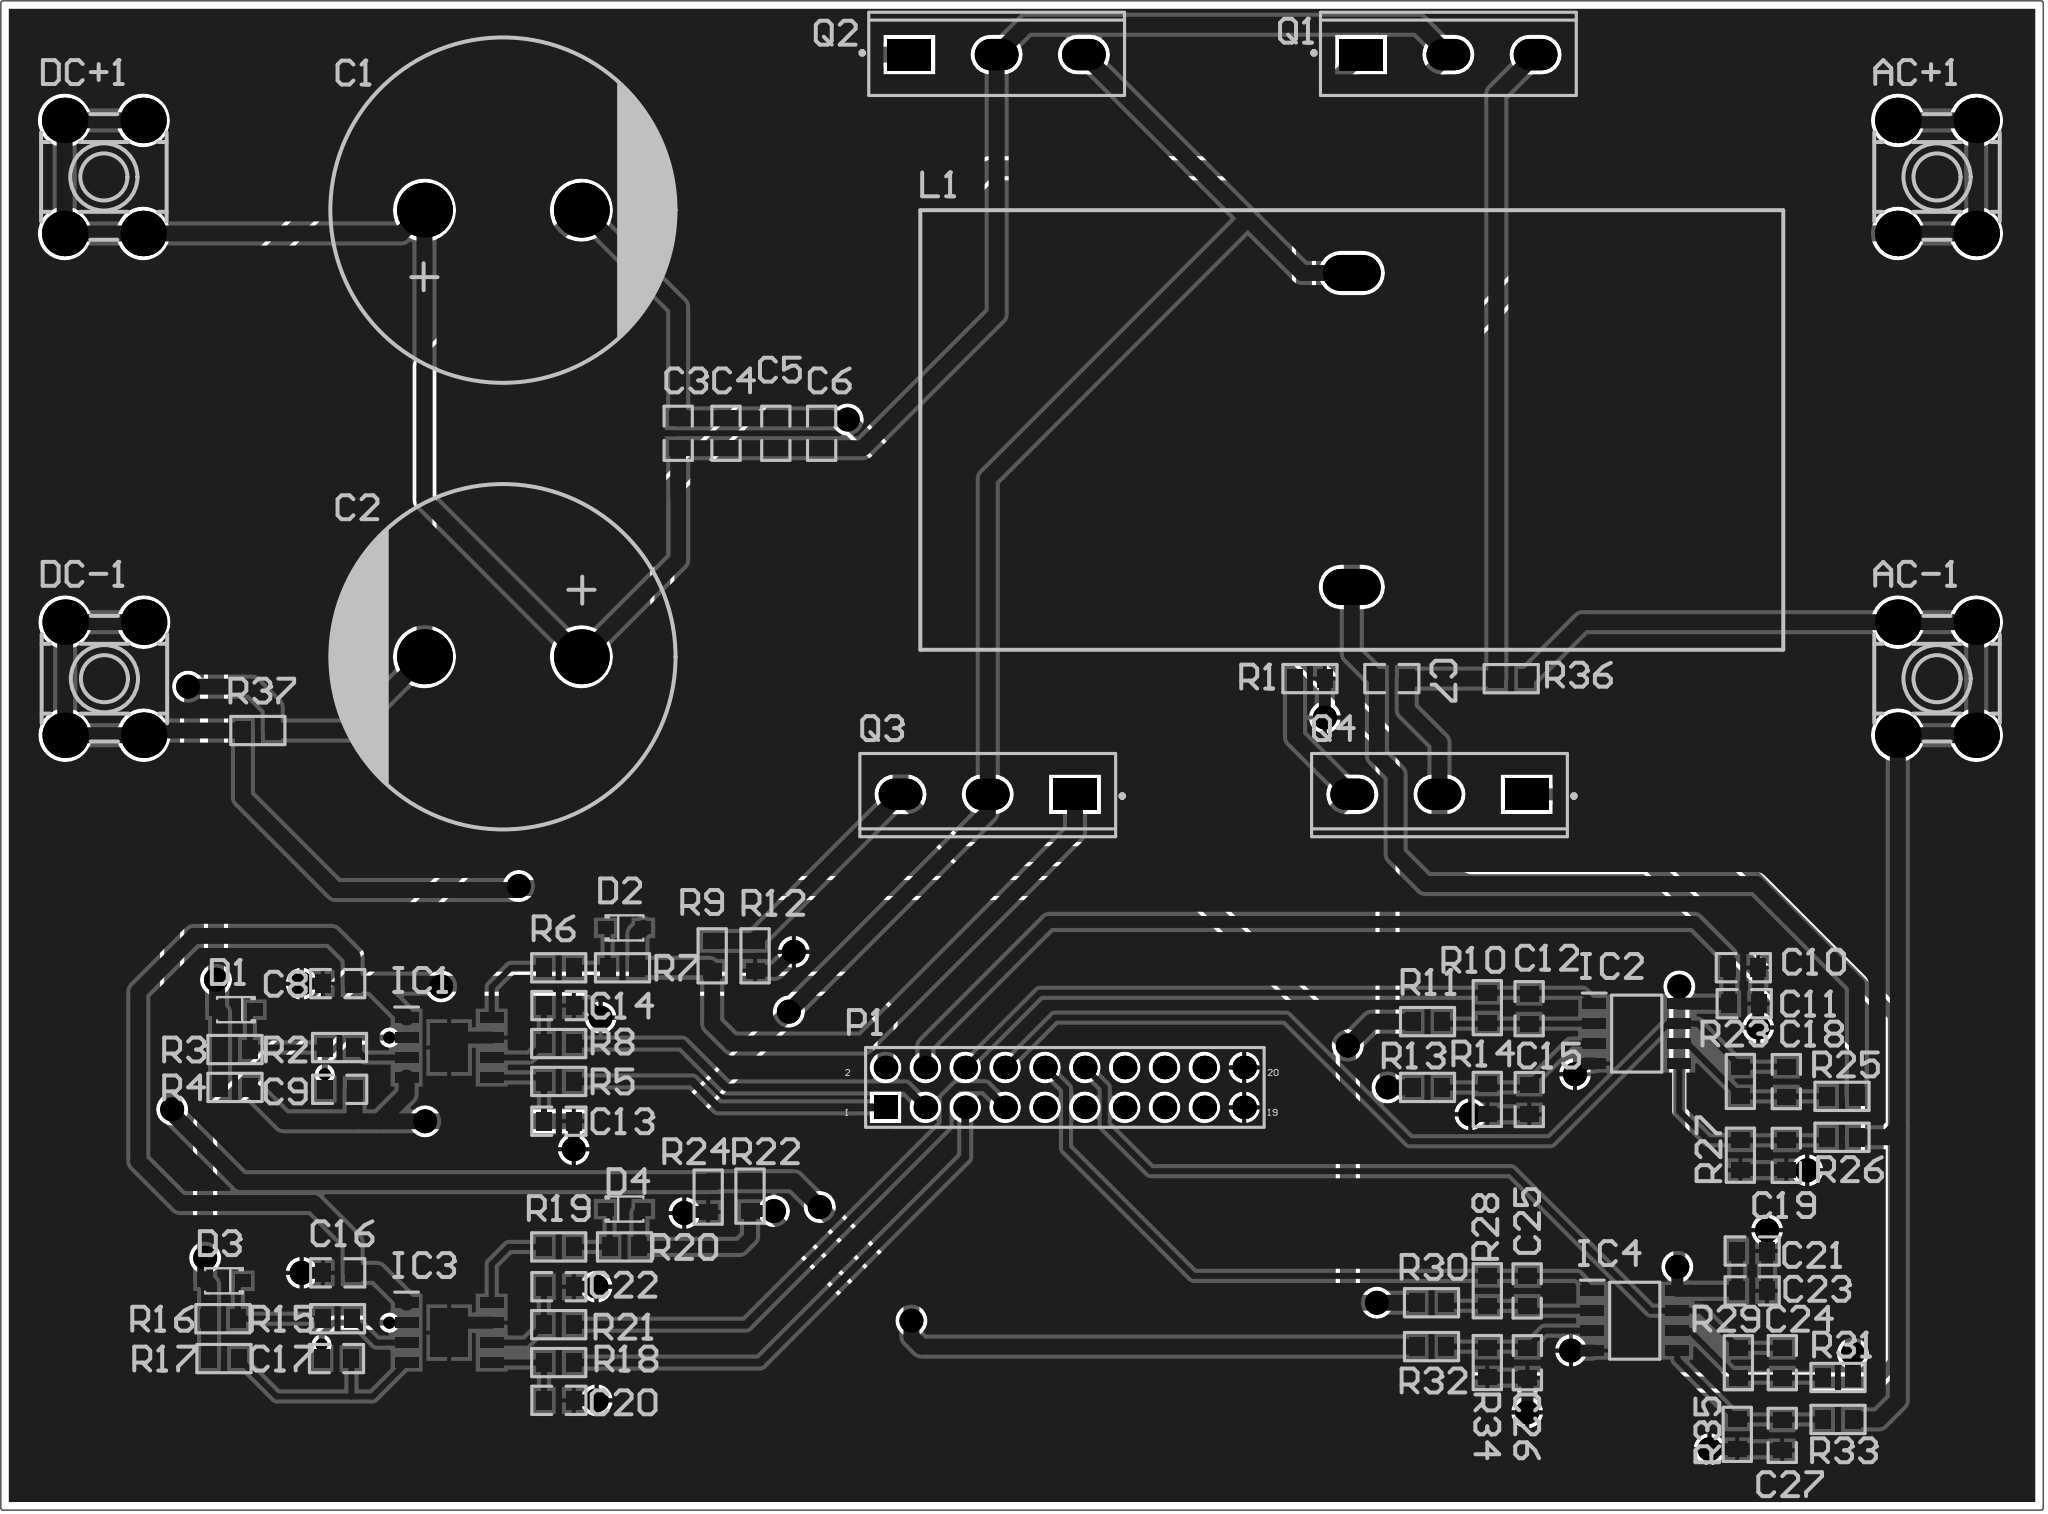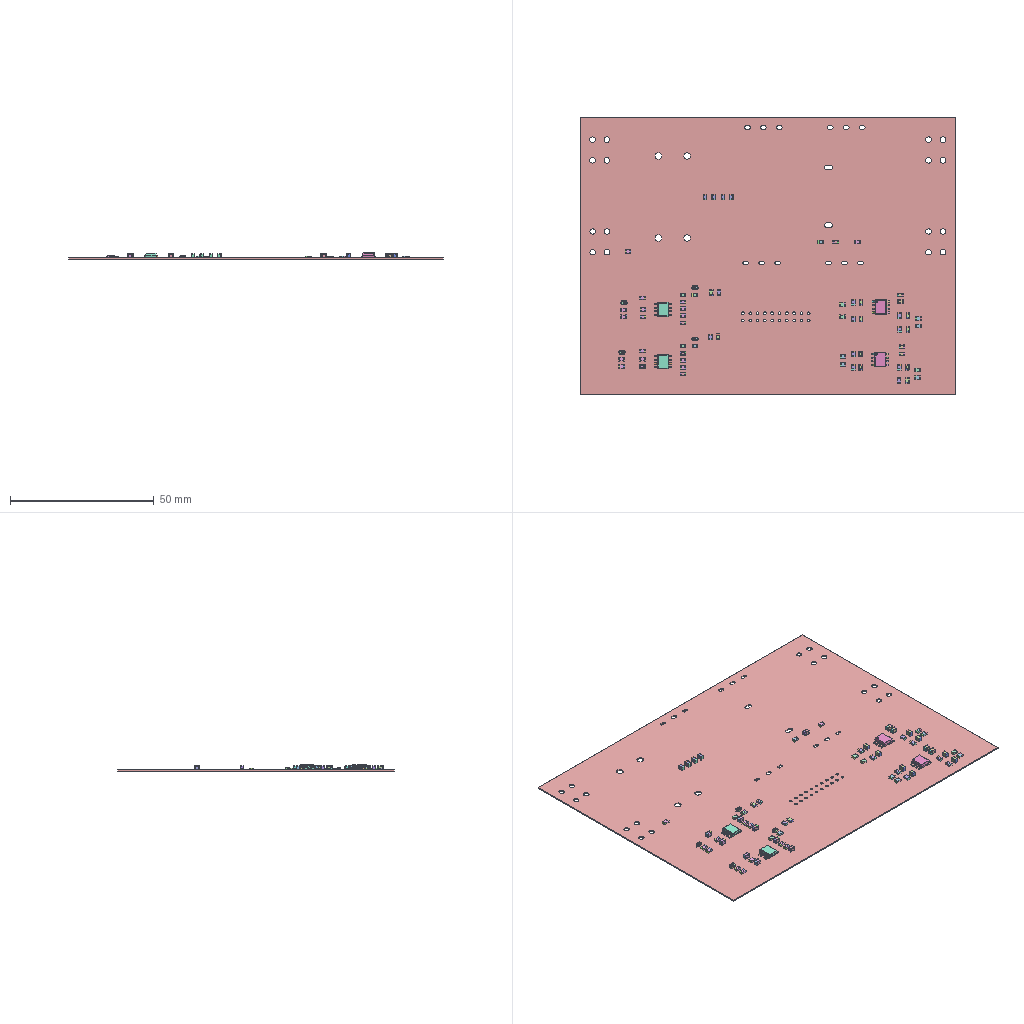Circuit board layout | Altium Designer | box 130.2 x 96.1 x 2.2 mm
Layer stack:
# Altium Designer layer stack of  (unit mm; dielectric type: 0 none, 1 core, 2 prepreg, 3 surface material)
index,name,kind,layer,copper_thickness_mm,dielectric_type,dielectric_thickness_mm,dielectric_material,dielectric_constant
0,Top Paste,other,,,,,,
1,Top Overlay,other,,,,,,
2,Top Solder,dielectric,,,3,0.0102,Solder Resist,3.5
3,Top Layer,copper,Top Layer,0.0356,,,,
4,Dielectric 1,dielectric,,,0,0.32,FR-4,4.8
5,Bottom Layer,copper,Bottom Layer,0.0356,,,,
6,Bottom Solder,dielectric,,,3,0.0102,Solder Resist,3.5
7,Bottom Overlay,other,,,,,,
8,Bottom Paste,other,,,,,,
# drill layer pairs: low layer,high layer
drill_pair,Top Layer,Bottom Layer
Part placement:
Designator,Comment,Layer,Footprint,Center-X(mm),Center-Y(mm),Rotation
R37,0R/1206,TopLayer,0805R,64.389,125.095,180
R36,0R/1206,TopLayer,0805R,144.272,128.397,180
R35,15k/0805,TopLayer,0805R,158.679,80.264,90
R34,15k/0805,TopLayer,0805R,142.748,84.836,90
R33,402k/0805,TopLayer,0805R,165.1,81.214,360
R32,402k/0805,TopLayer,0805R,139.192,85.852,360
R31,402k/0805,TopLayer,0805R,165.1,83.886,0
R30,402k/0805,TopLayer,0805R,139.192,88.646,360
R29,15k/0805,TopLayer,0805R,158.75,84.826,90
R28,15k/0805,TopLayer,0805R,142.748,89.408,90
R27,15k/0805,TopLayer,0805R,158.877,98.044,90
R26,402k/0805,TopLayer,0805R,165.354,99.187,360
R25,402k/0805,TopLayer,0805R,165.354,101.793,360
R24,1R/0603,TopLayer,0805R,93.091,95.377,90
R23,15k/0805,TopLayer,0805R,158.877,102.743,90
R22,10k/0603,TopLayer,0805R,95.758,95.438,270
R21,100R/0603,TopLayer,0805R,83.566,87.249,180
R20,2R/0603,TopLayer,0805R,87.757,92.202,360
R19,2R/0603,TopLayer,0805R,83.566,92.202,0
R18,100R/0603,TopLayer,0805R,83.566,84.836,180
R17,10k/0603,TopLayer,0805R,62.23,85.09,180
R16,2R/0603,TopLayer,0805R,62.164,87.63,180
R15,2R/0603,TopLayer,0805R,69.469,87.63,180
IC4,OPA2350UA,TopLayer,SOIC127P600X175-8N,152.146,87.503,0
IC3,UCC27211AQDDARQ1,TopLayer,SOIC8_Powerpad,76.581,86.741,0
D4,?,TopLayer,SOD-323,87.757,94.615,180
D3,?,TopLayer,SOD-323,62.23,90.043,0
C27,1nF/25V/0805,TopLayer,0805C,161.544,80.198,270
C26,1nF/25V/0805,TopLayer,0805C,145.302,84.826,270
C25,1nF/25V/0805,TopLayer,0805C,145.288,89.398,270
C24,1nF/25V/0805,TopLayer,0805C,161.551,84.826,270
C23,100nF/25V/0805,TopLayer,0805C,159.629,89.401,180
C22,100pF/25V/0603,TopLayer,0805C,83.576,89.669,360
C21,1nF/25V/0805,TopLayer,0805C,159.629,91.941,180
C20,100pF/25V/0603,TopLayer,0805C,83.576,82.43,360
C19,1nF/25V/0805,TopLayer,0805C,161.805,98.034,270
C18,1nF/25V/0805,TopLayer,0805C,161.805,102.733,270
C17,1uF/25V/0603,TopLayer,0805C,69.403,85.09,0
C16,1uF/25V/0603,TopLayer,0805C,69.479,90.551,0
R12,1R/0603,TopLayer,0805R,96.079,110.744,90
R14,15k/0805,TopLayer,0805R,142.748,101.6,90
R13,402k/0805,TopLayer,0805R,138.938,102.362,0
R11,402k/0805,TopLayer,0805R,138.938,106.553,0
R10,15k/0805,TopLayer,0805R,142.748,107.442,90
R1,0R/1206,TopLayer,0805R,131.445,128.404,360
R9,10k/0603,TopLayer,0805R,93.345,110.744,270
R8,100R/0603,TopLayer,0805R,83.566,105.156,180
R7,2R/0603,TopLayer,0805R,87.63,109.982,0
R6,2R/0603,TopLayer,0805R,83.566,109.982,0
R5,100R/0603,TopLayer,0805R,83.566,102.743,180
R4,10k/0603,TopLayer,0805R,62.931,102.362,180
R3,2R/0603,TopLayer,0805R,62.931,104.775,180
R2,2R/0603,TopLayer,0805R,69.596,104.902,180
Q4,IPW60R037CSFD,TopLayer,TO-247-3_L15.9-W5.1-P5.44-L,139.7,121.031,180
Q3,IPW60R037CSFD,TopLayer,TO-247-3_L15.9-W5.1-P5.44-L,110.91,121.031,180
Q2,IPW60R037CSFD,TopLayer,TO-247-3_L15.9-W5.1-P5.44-L,111.476,168.148,360
Q1,IPW60R037CSFD,TopLayer,TO-247-3_L15.9-W5.1-P5.44-L,140.266,168.148,360
P1,Header 10X2,TopLayer,HDR2X10,115.824,102.362,360
L1,Inductor,TopLayer,IND-TH_L55.0-W28.0-P20.00-D1.3,134.112,144.239,360
IC2,OPA2350UA,TopLayer,SOIC127P600X175-8N,152.273,105.791,0
IC1,UCC27211AQDDARQ1,TopLayer,SOIC8_Powerpad,76.581,104.902,0
DC-1,CONnector,TopLayer,CONN-TH_T44001,54.61,128.397,0
DC+1,CONnector,TopLayer,CONN-TH_T44001,54.575,160.357,180
D2,?,TopLayer,SOD-323,87.757,112.522,180
D1,?,TopLayer,SOD-323,62.992,107.315,0
C15,1nF/25V/0805,TopLayer,0805C,145.422,101.59,270
C12,1nF/25V/0805,TopLayer,0805C,145.415,107.376,270
C11,100nF/25V/0805,TopLayer,0805C,159.121,107.696,180
C10,1nF/25V/0805,TopLayer,0805C,159.065,109.989,180
C14,100pF/25V/0603,TopLayer,0805C,83.576,107.576,0
C13,100pF/25V/0603,TopLayer,0805C,83.576,100.21,360
C9,1uF/25V/0603,TopLayer,0805C,69.606,102.242,0
C8,1uF/25V/0603,TopLayer,0805C,69.479,108.973,0
C7,10uF/250V,TopLayer,0805C,136.662,128.404,360
C6,100nF/100V,TopLayer,0805C,100.323,144.028,90
C5,100nF/100V,TopLayer,0805C,97.402,144.028,90
C4,100nF/100V,TopLayer,0805C,94.227,144.028,90
C3,100nF/100V,TopLayer,0805C,91.179,144.028,90
C2,1000uF/100V,TopLayer,CAPE,80.01,129.794,180
C1,1000uF/100V,TopLayer,CAPE,80.01,158.242,0
AC-1,CONnector,TopLayer,CONN-TH_T44001,171.41,128.397,360
AC+1,CONnector,TopLayer,CONN-TH_T44001,171.41,160.357,0
Pad and via stacks:
# Altium Designer via and pad stacks of  (unit mm). Each distinct definition once, with the count of objects using it.
# via: kind,start_layer,end_layer,hole_mm,diameter_mm,mode(0 simple;1 top-mid-bottom;2 full stack),diameter_per_layer,count,example_net
# pad: kind,layer,hole_mm,hole_type(0 round;1 square;2 slot),plating,top_size,top_shape(1 round;2 rect;3 octagon;9 rounded rect),mid_size,bottom_size,mode,footprint,size_per_layer,count,example
pad,Multi-Layer,2.3,0,plated,3.5x3.5,1,3.5x3.5,3.5x3.5,0,CAPE,,4,C2.2
pad,Multi-Layer,1.2,2,plated,2x2.8,1,2x2.8,2x2.8,0,TO-247-3_L15.9-W5.1-P5.44-L,,8,Q1.3
pad,Multi-Layer,1.2,2,plated,2x2.8,2,2x2.8,2x2.8,0,TO-247-3_L15.9-W5.1-P5.44-L,,4,Q1.1
pad,Multi-Layer,1.9,0,plated,2.9x2.9,1,2.9x2.9,2.9x2.9,0,CONN-TH_T44001,,16,AC+1.0
pad,Multi-Layer,1.5,2,plated,3.7x2.3,1,3.7x2.3,3.7x2.3,0,IND-TH_L55.0-W28.0-P20.00-D1.3,,2,L1.1
pad,Multi-Layer,0.9,0,plated,1.5x1.5,1,1.5x1.5,1.5x1.5,0,HDR2X10,,19,P1.11
pad,Multi-Layer,0.9,0,plated,1.5x1.5,2,1.5x1.5,1.5x1.5,0,HDR2X10,,1,P1.1
pad,Top Layer,0,0,plated,1x1.2,2,1x1.2,1x1.2,0,0805C,,50,C10.2
pad,Top Layer,0,0,plated,1x1.2,2,1x1.2,1x1.2,0,0805R,,74,R13.1
pad,Top Layer,0,0,plated,1.525x0.65,2,1.525x0.65,1.525x0.65,0,SOIC127P600X175-8N,,16,IC2.8
pad,Top Layer,0,0,plated,1x0.8,2,1x0.8,1x0.8,0,SOD-323,,8,D3.2
pad,Top Layer,0,0,unplated,1.525x0.65,2,1.525x0.65,1.525x0.65,0,SOIC8 Powerpad,,16,IC3.1
pad,Top Layer,0,0,unplated,3.1x2.4,2,3.1x2.4,3.1x2.4,0,SOIC8 Powerpad,,2,IC3.9
via,Top Layer,Bottom Layer,0.762,1.524,0,,30,SGND
via,Top Layer,Bottom Layer,0.381,0.762,0,,4,NetC9_1
via,Top Layer,Bottom Layer,1.016,1.524,0,,7,IAC-
Copper pours:
name,layer,net,type(0 solid;1 hatched;2 none)
G,Top Layer,SGND,0
G,Bottom Layer,SGND,0
Design rules, without the lines most boards share:
# Altium Designer design rules of  (exported by Altium Designer, unit mm)
# columns: name | kind | enabled | priority | scope1 | scope2 | descriptor | typed fields (field=value)
SilkToSilkClearance | 55 | enabled | 1 | All | All | Silk to Silk (Clearance=0mil) (All),(All) |
SilkToSolderMaskClearance | 54 | enabled | 1 | IsPad | All | Silk To Solder Mask (Clearance=0mil) (IsPad),(All) |
MinimumSolderMaskSliver | 53 | enabled | 1 | All | All | Minimum Solder Mask Sliver (Gap=0mil) (All),(All) |
HoleToHoleClearance | 52 | enabled | 1 | All | All | Hole To Hole Clearance (Gap=10mil) (All),(All) | gap=0.254
DiffPairsRouting | 51 | enabled | 1 | All | All | Differential Pairs Uncoupled Length using the Gap Constraints (Min=10mil) (Max=10mil) (Prefered=10mil)  and Width Constraints (Min=15mil) (Max=15mil) (Prefered=15mil) (All) |
SolderMaskExpansion | 13 | enabled | 1 | All | All | Solder Mask Expansion (Expansion =4mil) (All) | expansion=0.1016
PasteMaskExpansion | 14 | enabled | 1 | All | All | Paste Mask Expansion (Expansion =0mil) (All) | expansion=0
RoutingVias | 11 | enabled | 1 | All | All | Routing Via (MinHoleWidth=28mil) (MaxHoleWidth=28mil) (PreferredHoleWidth=28mil) (MinWidth=50mil) (MaxWidth=50mil) (PreferedWidth=50mil) (All) | via_min_hole=0.7112 via_max_hole=0.7112 via_preferred_diameter=1.27 via_preferred_hole=0.7112
Width | 2 | enabled | 1 | All | All | Width Constraint (Min=10mil) (Max=60mil) (Preferred=10mil) (All) |
PolygonConnect | 20 | enabled | 1 | All | All | Polygon Connect Rule(Relief Connect )(Conductor Width=10mil) (Relief Angle=90 Angle) (Entries=4) (Air Gap Width=10mil) (All),(All) | connect_style(0=relief,1=direct,2=none)=0 relief_conductor_width=0.254 relief_entries=4
PlaneConnect | 6 | enabled | 1 | All | All | Power Plane Connect Rule(Relief Connect )(Expansion=20mil) (Conductor Width=10mil) (Air Gap=10mil) (Entries=4) (All) | relief_conductor_width=0.254 relief_entries=4 relief_expansion=0.508
Clearance | 0 | enabled | 1 | All | All | Clearance Constraint (Gap=10mil) (All),(All) | gap=0.254
Classes set for this board:
# Altium Designer classes of  (member kind: 0 net, 1 component, 2 from-to, 3 pad, 4 layer, 5 differential pair, 6 design channel, 7 polygon, 8 structure, 9 xSignal)
# columns: class name | member kind | superclass | members
Sheet1 | 1 | no | C1; C2; C3; C4; C5; C6; C7; C8; C9; C15; D1; D2; IC1; IC2; L1; P1; Q1; Q2; Q3; Q4; R10; R11; C16; C17; C18; C19; C20; C21; C22; C23; C24; C25; C26; C27; D3; D4; IC3; IC4; R14; R16; R17; R18; R19; R20; R21; R22; R23; R24; R25; R26; R27; R28; R29; R30; R31; R32; R33; R34; R35; R36; R37; C12; C14; R5; DC+1; R2; R9; R6; DC-1; R13; R3; R1; AC+1; C10; R7; R14; R4; AC-1; C11; C13; R8; R12;